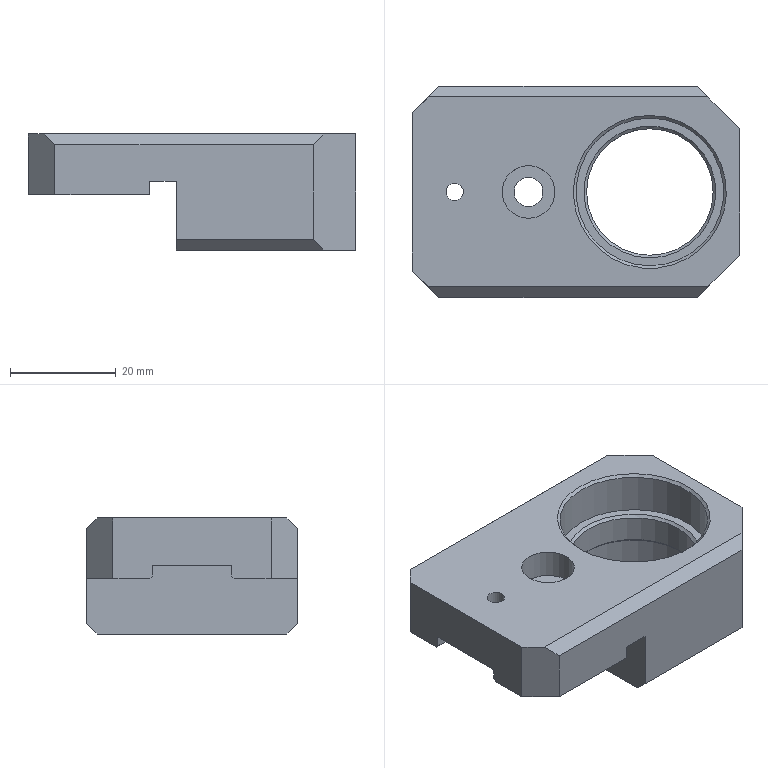Part | NX | 1 solid | 37 faces | box 62 x 40 x 22 mm | volume 26234 mm3 | plane 27 | cylinder 6 | cone 4 | commonest cylinder face diameters 28 x2 3.3 x1 5.5 x1 10 x1 24 x1
STEP:
#1=CARTESIAN_POINT('',(14.,-12.,-8.5));
#2=VERTEX_POINT('',#1);
#3=CARTESIAN_POINT('',(14.,0.,-8.5));
#4=DIRECTION('',(0.,0.,1.));
#5=DIRECTION('',(0.,-1.,0.));
#6=AXIS2_PLACEMENT_3D('',#3,#4,#5);
#7=CIRCLE('',#6,12.);
#8=EDGE_CURVE('',#2,#2,#7,.T.);
#9=ORIENTED_EDGE('',*,*,#8,.T.);
#10=EDGE_LOOP('',(#9));
#11=FACE_BOUND('',#10,.T.);
#12=CARTESIAN_POINT('',(14.,12.,-13.5));
#13=VERTEX_POINT('',#12);
#14=CARTESIAN_POINT('',(14.,0.,-13.5));
#15=DIRECTION('',(0.,0.,-1.));
#16=DIRECTION('',(0.,1.,0.));
#17=AXIS2_PLACEMENT_3D('',#14,#15,#16);
#18=CIRCLE('',#17,12.);
#19=EDGE_CURVE('',#13,#13,#18,.T.);
#20=ORIENTED_EDGE('',*,*,#19,.T.);
#21=EDGE_LOOP('',(#20));
#22=FACE_BOUND('',#21,.T.);
#23=CARTESIAN_POINT('',(14.,0.,-22.));
#24=DIRECTION('',(0.,0.,1.));
#25=DIRECTION('',(0.,-1.,0.));
#26=AXIS2_PLACEMENT_3D('',#23,#24,#25);
#27=CYLINDRICAL_SURFACE('',#26,12.);
#28=ADVANCED_FACE('',(#11,#22),#27,.F.);
#29=CARTESIAN_POINT('',(14.,-14.5,-22.));
#30=VERTEX_POINT('',#29);
#31=CARTESIAN_POINT('',(14.,0.,-22.));
#32=DIRECTION('',(0.,0.,1.));
#33=DIRECTION('',(0.,-1.,0.));
#34=AXIS2_PLACEMENT_3D('',#31,#32,#33);
#35=CIRCLE('',#34,14.5);
#36=EDGE_CURVE('',#30,#30,#35,.T.);
#37=ORIENTED_EDGE('',*,*,#36,.T.);
#38=EDGE_LOOP('',(#37));
#39=FACE_BOUND('',#38,.T.);
#40=CARTESIAN_POINT('',(31.,-12.,-22.));
#41=VERTEX_POINT('',#40);
#42=CARTESIAN_POINT('',(31.,12.,-22.));
#43=VERTEX_POINT('',#42);
#44=CARTESIAN_POINT('',(31.,-20.,-22.));
#45=DIRECTION('',(0.,1.,0.));
#46=VECTOR('',#45,1000.);
#47=LINE('',#44,#46);
#48=EDGE_CURVE('',#41,#43,#47,.T.);
#49=ORIENTED_EDGE('',*,*,#48,.F.);
#50=CARTESIAN_POINT('',(25.,-18.,-22.));
#51=VERTEX_POINT('',#50);
#52=CARTESIAN_POINT('',(31.,-12.,-22.));
#53=DIRECTION('',(0.7071,0.7071,0.));
#54=VECTOR('',#53,1000.);
#55=LINE('',#52,#54);
#56=EDGE_CURVE('',#41,#51,#55,.F.);
#57=ORIENTED_EDGE('',*,*,#56,.T.);
#58=CARTESIAN_POINT('',(-3.,-18.,-22.));
#59=VERTEX_POINT('',#58);
#60=CARTESIAN_POINT('',(31.,-18.,-22.));
#61=DIRECTION('',(-1.,0.,0.));
#62=VECTOR('',#61,1000.);
#63=LINE('',#60,#62);
#64=EDGE_CURVE('',#51,#59,#63,.T.);
#65=ORIENTED_EDGE('',*,*,#64,.T.);
#66=CARTESIAN_POINT('',(-3.,18.,-22.));
#67=VERTEX_POINT('',#66);
#68=CARTESIAN_POINT('',(-3.,-20.,-22.));
#69=DIRECTION('',(0.,-1.,0.));
#70=VECTOR('',#69,1000.);
#71=LINE('',#68,#70);
#72=EDGE_CURVE('',#67,#59,#71,.T.);
#73=ORIENTED_EDGE('',*,*,#72,.F.);
#74=CARTESIAN_POINT('',(25.,18.,-22.));
#75=VERTEX_POINT('',#74);
#76=CARTESIAN_POINT('',(31.,18.,-22.));
#77=DIRECTION('',(1.,0.,0.));
#78=VECTOR('',#77,1000.);
#79=LINE('',#76,#78);
#80=EDGE_CURVE('',#67,#75,#79,.T.);
#81=ORIENTED_EDGE('',*,*,#80,.T.);
#82=CARTESIAN_POINT('',(31.,12.,-22.));
#83=DIRECTION('',(-0.7071,0.7071,0.));
#84=VECTOR('',#83,1000.);
#85=LINE('',#82,#84);
#86=EDGE_CURVE('',#75,#43,#85,.F.);
#87=ORIENTED_EDGE('',*,*,#86,.T.);
#88=EDGE_LOOP('',(#49,#57,#65,#73,#81,#87));
#89=FACE_BOUND('',#88,.T.);
#90=CARTESIAN_POINT('',(31.,-20.,-22.));
#91=DIRECTION('',(0.,0.,1.));
#92=DIRECTION('',(0.,-1.,0.));
#93=AXIS2_PLACEMENT_3D('',#90,#91,#92);
#94=PLANE('',#93);
#95=ADVANCED_FACE('',(#39,#89),#94,.F.);
#96=CARTESIAN_POINT('',(23.,20.,-20.));
#97=VERTEX_POINT('',#96);
#98=CARTESIAN_POINT('',(-3.,20.,-20.));
#99=VERTEX_POINT('',#98);
#100=CARTESIAN_POINT('',(31.,20.,-20.));
#101=DIRECTION('',(-1.,0.,0.));
#102=VECTOR('',#101,1000.);
#103=LINE('',#100,#102);
#104=EDGE_CURVE('',#97,#99,#103,.T.);
#105=ORIENTED_EDGE('',*,*,#104,.F.);
#106=CARTESIAN_POINT('',(25.667,17.333,-22.667));
#107=DIRECTION('',(0.5774,-0.5774,-0.5774));
#108=VECTOR('',#107,1000.);
#109=LINE('',#106,#108);
#110=EDGE_CURVE('',#97,#75,#109,.T.);
#111=ORIENTED_EDGE('',*,*,#110,.T.);
#112=ORIENTED_EDGE('',*,*,#80,.F.);
#113=CARTESIAN_POINT('',(-3.,20.,-20.));
#114=DIRECTION('',(0.,-0.7071,-0.7071));
#115=VECTOR('',#114,1000.);
#116=LINE('',#113,#115);
#117=EDGE_CURVE('',#67,#99,#116,.F.);
#118=ORIENTED_EDGE('',*,*,#117,.T.);
#119=EDGE_LOOP('',(#105,#111,#112,#118));
#120=FACE_BOUND('',#119,.T.);
#121=CARTESIAN_POINT('',(31.,20.,-20.));
#122=DIRECTION('',(0.,-0.7071,0.7071));
#123=DIRECTION('',(-1.,0.,0.));
#124=AXIS2_PLACEMENT_3D('',#121,#122,#123);
#125=PLANE('',#124);
#126=ADVANCED_FACE('',(#120),#125,.F.);
#127=ORIENTED_EDGE('',*,*,#64,.F.);
#128=CARTESIAN_POINT('',(23.,-20.,-20.));
#129=VERTEX_POINT('',#128);
#130=CARTESIAN_POINT('',(27.,-16.,-24.));
#131=DIRECTION('',(-0.5774,-0.5774,0.5774));
#132=VECTOR('',#131,1000.);
#133=LINE('',#130,#132);
#134=EDGE_CURVE('',#51,#129,#133,.T.);
#135=ORIENTED_EDGE('',*,*,#134,.T.);
#136=CARTESIAN_POINT('',(-3.,-20.,-20.));
#137=VERTEX_POINT('',#136);
#138=CARTESIAN_POINT('',(31.,-20.,-20.));
#139=DIRECTION('',(1.,0.,0.));
#140=VECTOR('',#139,1000.);
#141=LINE('',#138,#140);
#142=EDGE_CURVE('',#137,#129,#141,.T.);
#143=ORIENTED_EDGE('',*,*,#142,.F.);
#144=CARTESIAN_POINT('',(-3.,-18.,-22.));
#145=DIRECTION('',(0.,-0.7071,0.7071));
#146=VECTOR('',#145,1000.);
#147=LINE('',#144,#146);
#148=EDGE_CURVE('',#137,#59,#147,.F.);
#149=ORIENTED_EDGE('',*,*,#148,.T.);
#150=EDGE_LOOP('',(#127,#135,#143,#149));
#151=FACE_BOUND('',#150,.T.);
#152=CARTESIAN_POINT('',(31.,-18.,-22.));
#153=DIRECTION('',(0.,0.7071,0.7071));
#154=DIRECTION('',(-1.,0.,0.));
#155=AXIS2_PLACEMENT_3D('',#152,#153,#154);
#156=PLANE('',#155);
#157=ADVANCED_FACE('',(#151),#156,.F.);
#158=CARTESIAN_POINT('',(-31.,-7.5,-9.));
#159=VERTEX_POINT('',#158);
#160=CARTESIAN_POINT('',(-31.,-7.5,-11.));
#161=VERTEX_POINT('',#160);
#162=CARTESIAN_POINT('',(-31.,-7.5,-35.));
#163=DIRECTION('',(0.,0.,-1.));
#164=VECTOR('',#163,1000.);
#165=LINE('',#162,#164);
#166=EDGE_CURVE('',#159,#161,#165,.T.);
#167=ORIENTED_EDGE('',*,*,#166,.T.);
#168=CARTESIAN_POINT('',(-31.,-8.,-11.5));
#169=VERTEX_POINT('',#168);
#170=CARTESIAN_POINT('',(-31.,-3.75,-7.25));
#171=DIRECTION('',(0.,-0.7071,-0.7071));
#172=VECTOR('',#171,1000.);
#173=LINE('',#170,#172);
#174=EDGE_CURVE('',#161,#169,#173,.T.);
#175=ORIENTED_EDGE('',*,*,#174,.T.);
#176=CARTESIAN_POINT('',(-31.,-15.,-11.5));
#177=VERTEX_POINT('',#176);
#178=CARTESIAN_POINT('',(-31.,-20.,-11.5));
#179=DIRECTION('',(0.,1.,0.));
#180=VECTOR('',#179,1000.);
#181=LINE('',#178,#180);
#182=EDGE_CURVE('',#177,#169,#181,.T.);
#183=ORIENTED_EDGE('',*,*,#182,.F.);
#184=CARTESIAN_POINT('',(-31.,-15.,0.));
#185=VERTEX_POINT('',#184);
#186=CARTESIAN_POINT('',(-31.,-15.,-2.));
#187=DIRECTION('',(0.,0.,1.));
#188=VECTOR('',#187,1000.);
#189=LINE('',#186,#188);
#190=EDGE_CURVE('',#177,#185,#189,.T.);
#191=ORIENTED_EDGE('',*,*,#190,.T.);
#192=CARTESIAN_POINT('',(-31.,15.,0.));
#193=VERTEX_POINT('',#192);
#194=CARTESIAN_POINT('',(-31.,-20.,0.));
#195=DIRECTION('',(0.,-1.,0.));
#196=VECTOR('',#195,1000.);
#197=LINE('',#194,#196);
#198=EDGE_CURVE('',#193,#185,#197,.T.);
#199=ORIENTED_EDGE('',*,*,#198,.F.);
#200=CARTESIAN_POINT('',(-31.,15.,-11.5));
#201=VERTEX_POINT('',#200);
#202=CARTESIAN_POINT('',(-31.,15.,-13.5));
#203=DIRECTION('',(0.,0.,-1.));
#204=VECTOR('',#203,1000.);
#205=LINE('',#202,#204);
#206=EDGE_CURVE('',#193,#201,#205,.T.);
#207=ORIENTED_EDGE('',*,*,#206,.T.);
#208=CARTESIAN_POINT('',(-31.,8.,-11.5));
#209=VERTEX_POINT('',#208);
#210=CARTESIAN_POINT('',(-31.,-20.,-11.5));
#211=DIRECTION('',(0.,1.,0.));
#212=VECTOR('',#211,1000.);
#213=LINE('',#210,#212);
#214=EDGE_CURVE('',#209,#201,#213,.T.);
#215=ORIENTED_EDGE('',*,*,#214,.F.);
#216=CARTESIAN_POINT('',(-31.,7.5,-11.));
#217=VERTEX_POINT('',#216);
#218=CARTESIAN_POINT('',(-31.,3.75,-7.25));
#219=DIRECTION('',(0.,-0.7071,0.7071));
#220=VECTOR('',#219,1000.);
#221=LINE('',#218,#220);
#222=EDGE_CURVE('',#209,#217,#221,.T.);
#223=ORIENTED_EDGE('',*,*,#222,.T.);
#224=CARTESIAN_POINT('',(-31.,7.5,-9.));
#225=VERTEX_POINT('',#224);
#226=CARTESIAN_POINT('',(-31.,7.5,-11.));
#227=DIRECTION('',(0.,0.,1.));
#228=VECTOR('',#227,1000.);
#229=LINE('',#226,#228);
#230=EDGE_CURVE('',#217,#225,#229,.T.);
#231=ORIENTED_EDGE('',*,*,#230,.T.);
#232=CARTESIAN_POINT('',(-31.,-7.5,-9.));
#233=DIRECTION('',(0.,-1.,0.));
#234=VECTOR('',#233,1000.);
#235=LINE('',#232,#234);
#236=EDGE_CURVE('',#225,#159,#235,.T.);
#237=ORIENTED_EDGE('',*,*,#236,.T.);
#238=EDGE_LOOP('',(#167,#175,#183,#191,#199,#207,#215,#223,#231,#237));
#239=FACE_BOUND('',#238,.T.);
#240=CARTESIAN_POINT('',(-31.,0.,-11.));
#241=DIRECTION('',(-1.,0.,0.));
#242=DIRECTION('',(0.,0.,1.));
#243=AXIS2_PLACEMENT_3D('',#240,#241,#242);
#244=PLANE('',#243);
#245=ADVANCED_FACE('',(#239),#244,.T.);
#246=CARTESIAN_POINT('',(-8.,20.,-9.));
#247=VERTEX_POINT('',#246);
#248=CARTESIAN_POINT('',(-8.,20.,-11.5));
#249=VERTEX_POINT('',#248);
#250=CARTESIAN_POINT('',(-8.,20.,31.311));
#251=DIRECTION('',(0.,0.,-1.));
#252=VECTOR('',#251,1000.);
#253=LINE('',#250,#252);
#254=EDGE_CURVE('',#247,#249,#253,.T.);
#255=ORIENTED_EDGE('',*,*,#254,.T.);
#256=CARTESIAN_POINT('',(-26.,20.,-11.5));
#257=VERTEX_POINT('',#256);
#258=CARTESIAN_POINT('',(37.112,20.,-11.5));
#259=DIRECTION('',(-1.,0.,0.));
#260=VECTOR('',#259,1000.);
#261=LINE('',#258,#260);
#262=EDGE_CURVE('',#249,#257,#261,.T.);
#263=ORIENTED_EDGE('',*,*,#262,.T.);
#264=CARTESIAN_POINT('',(-26.,20.,-2.));
#265=VERTEX_POINT('',#264);
#266=CARTESIAN_POINT('',(-26.,20.,-2.));
#267=DIRECTION('',(0.,0.,1.));
#268=VECTOR('',#267,1000.);
#269=LINE('',#266,#268);
#270=EDGE_CURVE('',#257,#265,#269,.T.);
#271=ORIENTED_EDGE('',*,*,#270,.T.);
#272=CARTESIAN_POINT('',(23.,20.,-2.));
#273=VERTEX_POINT('',#272);
#274=CARTESIAN_POINT('',(31.,20.,-2.));
#275=DIRECTION('',(1.,0.,0.));
#276=VECTOR('',#275,1000.);
#277=LINE('',#274,#276);
#278=EDGE_CURVE('',#265,#273,#277,.T.);
#279=ORIENTED_EDGE('',*,*,#278,.T.);
#280=CARTESIAN_POINT('',(23.,20.,-22.));
#281=DIRECTION('',(0.,0.,-1.));
#282=VECTOR('',#281,1000.);
#283=LINE('',#280,#282);
#284=EDGE_CURVE('',#273,#97,#283,.T.);
#285=ORIENTED_EDGE('',*,*,#284,.T.);
#286=ORIENTED_EDGE('',*,*,#104,.T.);
#287=CARTESIAN_POINT('',(-3.,20.,-9.));
#288=VERTEX_POINT('',#287);
#289=CARTESIAN_POINT('',(-3.,20.,-14.));
#290=DIRECTION('',(0.,0.,1.));
#291=VECTOR('',#290,1000.);
#292=LINE('',#289,#291);
#293=EDGE_CURVE('',#99,#288,#292,.T.);
#294=ORIENTED_EDGE('',*,*,#293,.T.);
#295=CARTESIAN_POINT('',(-3.,20.,-9.));
#296=DIRECTION('',(-1.,0.,0.));
#297=VECTOR('',#296,1000.);
#298=LINE('',#295,#297);
#299=EDGE_CURVE('',#288,#247,#298,.T.);
#300=ORIENTED_EDGE('',*,*,#299,.T.);
#301=EDGE_LOOP('',(#255,#263,#271,#279,#285,#286,#294,#300));
#302=FACE_BOUND('',#301,.T.);
#303=CARTESIAN_POINT('',(31.,20.,-22.));
#304=DIRECTION('',(0.,-1.,0.));
#305=DIRECTION('',(0.,0.,-1.));
#306=AXIS2_PLACEMENT_3D('',#303,#304,#305);
#307=PLANE('',#306);
#308=ADVANCED_FACE('',(#302),#307,.F.);
#309=CARTESIAN_POINT('',(-9.,-5.,0.));
#310=VERTEX_POINT('',#309);
#311=CARTESIAN_POINT('',(-9.,0.,0.));
#312=DIRECTION('',(0.,0.,1.));
#313=DIRECTION('',(0.,-1.,0.));
#314=AXIS2_PLACEMENT_3D('',#311,#312,#313);
#315=CIRCLE('',#314,5.);
#316=EDGE_CURVE('',#310,#310,#315,.T.);
#317=ORIENTED_EDGE('',*,*,#316,.F.);
#318=EDGE_LOOP('',(#317));
#319=FACE_BOUND('',#318,.T.);
#320=CARTESIAN_POINT('',(14.,14.5,0.));
#321=VERTEX_POINT('',#320);
#322=CARTESIAN_POINT('',(14.,0.,0.));
#323=DIRECTION('',(0.,0.,-1.));
#324=DIRECTION('',(0.,1.,0.));
#325=AXIS2_PLACEMENT_3D('',#322,#323,#324);
#326=CIRCLE('',#325,14.5);
#327=EDGE_CURVE('',#321,#321,#326,.T.);
#328=ORIENTED_EDGE('',*,*,#327,.T.);
#329=EDGE_LOOP('',(#328));
#330=FACE_BOUND('',#329,.T.);
#331=CARTESIAN_POINT('',(-23.,1.65,0.));
#332=VERTEX_POINT('',#331);
#333=CARTESIAN_POINT('',(-23.,0.,0.));
#334=DIRECTION('',(0.,0.,-1.));
#335=DIRECTION('',(0.,1.,0.));
#336=AXIS2_PLACEMENT_3D('',#333,#334,#335);
#337=CIRCLE('',#336,1.65);
#338=EDGE_CURVE('',#332,#332,#337,.T.);
#339=ORIENTED_EDGE('',*,*,#338,.T.);
#340=EDGE_LOOP('',(#339));
#341=FACE_BOUND('',#340,.T.);
#342=ORIENTED_EDGE('',*,*,#198,.T.);
#343=CARTESIAN_POINT('',(-28.,-18.,0.));
#344=VERTEX_POINT('',#343);
#345=CARTESIAN_POINT('',(-26.,-20.,0.));
#346=DIRECTION('',(0.7071,-0.7071,0.));
#347=VECTOR('',#346,1000.);
#348=LINE('',#345,#347);
#349=EDGE_CURVE('',#185,#344,#348,.T.);
#350=ORIENTED_EDGE('',*,*,#349,.T.);
#351=CARTESIAN_POINT('',(25.,-18.,0.));
#352=VERTEX_POINT('',#351);
#353=CARTESIAN_POINT('',(31.,-18.,0.));
#354=DIRECTION('',(1.,0.,0.));
#355=VECTOR('',#354,1000.);
#356=LINE('',#353,#355);
#357=EDGE_CURVE('',#344,#352,#356,.T.);
#358=ORIENTED_EDGE('',*,*,#357,.T.);
#359=CARTESIAN_POINT('',(31.,-12.,0.));
#360=VERTEX_POINT('',#359);
#361=CARTESIAN_POINT('',(31.,-12.,0.));
#362=DIRECTION('',(-0.7071,-0.7071,0.));
#363=VECTOR('',#362,1000.);
#364=LINE('',#361,#363);
#365=EDGE_CURVE('',#352,#360,#364,.F.);
#366=ORIENTED_EDGE('',*,*,#365,.T.);
#367=CARTESIAN_POINT('',(31.,12.,0.));
#368=VERTEX_POINT('',#367);
#369=CARTESIAN_POINT('',(31.,-20.,0.));
#370=DIRECTION('',(0.,-1.,0.));
#371=VECTOR('',#370,1000.);
#372=LINE('',#369,#371);
#373=EDGE_CURVE('',#368,#360,#372,.T.);
#374=ORIENTED_EDGE('',*,*,#373,.F.);
#375=CARTESIAN_POINT('',(25.,18.,0.));
#376=VERTEX_POINT('',#375);
#377=CARTESIAN_POINT('',(31.,12.,0.));
#378=DIRECTION('',(0.7071,-0.7071,0.));
#379=VECTOR('',#378,1000.);
#380=LINE('',#377,#379);
#381=EDGE_CURVE('',#368,#376,#380,.F.);
#382=ORIENTED_EDGE('',*,*,#381,.T.);
#383=CARTESIAN_POINT('',(-28.,18.,0.));
#384=VERTEX_POINT('',#383);
#385=CARTESIAN_POINT('',(31.,18.,0.));
#386=DIRECTION('',(-1.,0.,0.));
#387=VECTOR('',#386,1000.);
#388=LINE('',#385,#387);
#389=EDGE_CURVE('',#376,#384,#388,.T.);
#390=ORIENTED_EDGE('',*,*,#389,.T.);
#391=CARTESIAN_POINT('',(-26.,20.,0.));
#392=DIRECTION('',(-0.7071,-0.7071,0.));
#393=VECTOR('',#392,1000.);
#394=LINE('',#391,#393);
#395=EDGE_CURVE('',#384,#193,#394,.T.);
#396=ORIENTED_EDGE('',*,*,#395,.T.);
#397=EDGE_LOOP('',(#342,#350,#358,#366,#374,#382,#390,#396));
#398=FACE_BOUND('',#397,.T.);
#399=CARTESIAN_POINT('',(31.,-20.,0.));
#400=DIRECTION('',(0.,0.,-1.));
#401=DIRECTION('',(0.,1.,0.));
#402=AXIS2_PLACEMENT_3D('',#399,#400,#401);
#403=PLANE('',#402);
#404=ADVANCED_FACE('',(#319,#330,#341,#398),#403,.F.);
#405=CARTESIAN_POINT('',(-26.,-20.,-2.));
#406=VERTEX_POINT('',#405);
#407=CARTESIAN_POINT('',(-26.,-20.,-11.5));
#408=VERTEX_POINT('',#407);
#409=CARTESIAN_POINT('',(-26.,-20.,-13.5));
#410=DIRECTION('',(0.,0.,-1.));
#411=VECTOR('',#410,1000.);
#412=LINE('',#409,#411);
#413=EDGE_CURVE('',#406,#408,#412,.T.);
#414=ORIENTED_EDGE('',*,*,#413,.T.);
#415=CARTESIAN_POINT('',(-8.,-20.,-11.5));
#416=VERTEX_POINT('',#415);
#417=CARTESIAN_POINT('',(37.112,-20.,-11.5));
#418=DIRECTION('',(-1.,0.,0.));
#419=VECTOR('',#418,1000.);
#420=LINE('',#417,#419);
#421=EDGE_CURVE('',#416,#408,#420,.T.);
#422=ORIENTED_EDGE('',*,*,#421,.F.);
#423=CARTESIAN_POINT('',(-8.,-20.,-9.));
#424=VERTEX_POINT('',#423);
#425=CARTESIAN_POINT('',(-8.,-20.,31.311));
#426=DIRECTION('',(0.,0.,-1.));
#427=VECTOR('',#426,1000.);
#428=LINE('',#425,#427);
#429=EDGE_CURVE('',#424,#416,#428,.T.);
#430=ORIENTED_EDGE('',*,*,#429,.F.);
#431=CARTESIAN_POINT('',(-3.,-20.,-9.));
#432=VERTEX_POINT('',#431);
#433=CARTESIAN_POINT('',(-3.,-20.,-9.));
#434=DIRECTION('',(1.,0.,0.));
#435=VECTOR('',#434,1000.);
#436=LINE('',#433,#435);
#437=EDGE_CURVE('',#424,#432,#436,.T.);
#438=ORIENTED_EDGE('',*,*,#437,.T.);
#439=CARTESIAN_POINT('',(-3.,-20.,-14.));
#440=DIRECTION('',(0.,0.,-1.));
#441=VECTOR('',#440,1000.);
#442=LINE('',#439,#441);
#443=EDGE_CURVE('',#432,#137,#442,.T.);
#444=ORIENTED_EDGE('',*,*,#443,.T.);
#445=ORIENTED_EDGE('',*,*,#142,.T.);
#446=CARTESIAN_POINT('',(23.,-20.,-2.));
#447=VERTEX_POINT('',#446);
#448=CARTESIAN_POINT('',(23.,-20.,-22.));
#449=DIRECTION('',(0.,0.,1.));
#450=VECTOR('',#449,1000.);
#451=LINE('',#448,#450);
#452=EDGE_CURVE('',#129,#447,#451,.T.);
#453=ORIENTED_EDGE('',*,*,#452,.T.);
#454=CARTESIAN_POINT('',(31.,-20.,-2.));
#455=DIRECTION('',(-1.,0.,0.));
#456=VECTOR('',#455,1000.);
#457=LINE('',#454,#456);
#458=EDGE_CURVE('',#447,#406,#457,.T.);
#459=ORIENTED_EDGE('',*,*,#458,.T.);
#460=EDGE_LOOP('',(#414,#422,#430,#438,#444,#445,#453,#459));
#461=FACE_BOUND('',#460,.T.);
#462=CARTESIAN_POINT('',(31.,-20.,-22.));
#463=DIRECTION('',(0.,1.,0.));
#464=DIRECTION('',(0.,0.,1.));
#465=AXIS2_PLACEMENT_3D('',#462,#463,#464);
#466=PLANE('',#465);
#467=ADVANCED_FACE('',(#461),#466,.F.);
#468=ORIENTED_EDGE('',*,*,#373,.T.);
#469=CARTESIAN_POINT('',(31.,-12.,-11.));
#470=DIRECTION('',(0.,0.,-1.));
#471=VECTOR('',#470,1000.);
#472=LINE('',#469,#471);
#473=EDGE_CURVE('',#360,#41,#472,.T.);
#474=ORIENTED_EDGE('',*,*,#473,.T.);
#475=ORIENTED_EDGE('',*,*,#48,.T.);
#476=CARTESIAN_POINT('',(31.,12.,-11.));
#477=DIRECTION('',(0.,0.,1.));
#478=VECTOR('',#477,1000.);
#479=LINE('',#476,#478);
#480=EDGE_CURVE('',#43,#368,#479,.T.);
#481=ORIENTED_EDGE('',*,*,#480,.T.);
#482=EDGE_LOOP('',(#468,#474,#475,#481));
#483=FACE_BOUND('',#482,.T.);
#484=CARTESIAN_POINT('',(31.,0.,-11.));
#485=DIRECTION('',(-1.,0.,0.));
#486=DIRECTION('',(0.,0.,1.));
#487=AXIS2_PLACEMENT_3D('',#484,#485,#486);
#488=PLANE('',#487);
#489=ADVANCED_FACE('',(#483),#488,.F.);
#490=ORIENTED_EDGE('',*,*,#357,.F.);
#491=CARTESIAN_POINT('',(-7.,-39.,-21.));
#492=DIRECTION('',(-0.5774,0.5774,0.5774));
#493=VECTOR('',#492,1000.);
#494=LINE('',#491,#493);
#495=EDGE_CURVE('',#344,#406,#494,.F.);
#496=ORIENTED_EDGE('',*,*,#495,.T.);
#497=ORIENTED_EDGE('',*,*,#458,.F.);
#498=CARTESIAN_POINT('',(25.667,-17.333,0.6667));
#499=DIRECTION('',(0.5774,0.5774,0.5774));
#500=VECTOR('',#499,1000.);
#501=LINE('',#498,#500);
#502=EDGE_CURVE('',#447,#352,#501,.T.);
#503=ORIENTED_EDGE('',*,*,#502,.T.);
#504=EDGE_LOOP('',(#490,#496,#497,#503));
#505=FACE_BOUND('',#504,.T.);
#506=CARTESIAN_POINT('',(31.,-20.,-2.));
#507=DIRECTION('',(0.,0.7071,-0.7071));
#508=DIRECTION('',(-1.,0.,0.));
#509=AXIS2_PLACEMENT_3D('',#506,#507,#508);
#510=PLANE('',#509);
#511=ADVANCED_FACE('',(#505),#510,.F.);
#512=ORIENTED_EDGE('',*,*,#278,.F.);
#513=CARTESIAN_POINT('',(-8.333,37.667,-19.667));
#514=DIRECTION('',(0.5774,0.5774,-0.5774));
#515=VECTOR('',#514,1000.);
#516=LINE('',#513,#515);
#517=EDGE_CURVE('',#265,#384,#516,.F.);
#518=ORIENTED_EDGE('',*,*,#517,.T.);
#519=ORIENTED_EDGE('',*,*,#389,.F.);
#520=CARTESIAN_POINT('',(27.,16.,2.));
#521=DIRECTION('',(-0.5774,0.5774,-0.5774));
#522=VECTOR('',#521,1000.);
#523=LINE('',#520,#522);
#524=EDGE_CURVE('',#376,#273,#523,.T.);
#525=ORIENTED_EDGE('',*,*,#524,.T.);
#526=EDGE_LOOP('',(#512,#518,#519,#525));
#527=FACE_BOUND('',#526,.T.);
#528=CARTESIAN_POINT('',(31.,18.,0.));
#529=DIRECTION('',(0.,-0.7071,-0.7071));
#530=DIRECTION('',(-1.,0.,0.));
#531=AXIS2_PLACEMENT_3D('',#528,#529,#530);
#532=PLANE('',#531);
#533=ADVANCED_FACE('',(#527),#532,.F.);
#534=CARTESIAN_POINT('',(-3.,-7.5,-9.));
#535=DIRECTION('',(0.,-1.,0.));
#536=VECTOR('',#535,1000.);
#537=LINE('',#534,#536);
#538=EDGE_CURVE('',#288,#432,#537,.T.);
#539=ORIENTED_EDGE('',*,*,#538,.F.);
#540=ORIENTED_EDGE('',*,*,#293,.F.);
#541=ORIENTED_EDGE('',*,*,#117,.F.);
#542=ORIENTED_EDGE('',*,*,#72,.T.);
#543=ORIENTED_EDGE('',*,*,#148,.F.);
#544=ORIENTED_EDGE('',*,*,#443,.F.);
#545=EDGE_LOOP('',(#539,#540,#541,#542,#543,#544));
#546=FACE_BOUND('',#545,.T.);
#547=CARTESIAN_POINT('',(-3.,0.,-11.));
#548=DIRECTION('',(-1.,0.,0.));
#549=DIRECTION('',(0.,0.,1.));
#550=AXIS2_PLACEMENT_3D('',#547,#548,#549);
#551=PLANE('',#550);
#552=ADVANCED_FACE('',(#546),#551,.T.);
#553=ORIENTED_EDGE('',*,*,#230,.F.);
#554=CARTESIAN_POINT('',(-8.,7.5,-11.));
#555=VERTEX_POINT('',#554);
#556=CARTESIAN_POINT('',(-8.,7.5,-11.));
#557=DIRECTION('',(1.,0.,0.));
#558=VECTOR('',#557,1000.);
#559=LINE('',#556,#558);
#560=EDGE_CURVE('',#217,#555,#559,.T.);
#561=ORIENTED_EDGE('',*,*,#560,.T.);
#562=CARTESIAN_POINT('',(-8.,7.5,-9.));
#563=VERTEX_POINT('',#562);
#564=CARTESIAN_POINT('',(-8.,7.5,-35.));
#565=DIRECTION('',(0.,0.,-1.));
#566=VECTOR('',#565,1000.);
#567=LINE('',#564,#566);
#568=EDGE_CURVE('',#563,#555,#567,.T.);
#569=ORIENTED_EDGE('',*,*,#568,.F.);
#570=CARTESIAN_POINT('',(-3.,7.5,-9.));
#571=DIRECTION('',(-1.,0.,0.));
#572=VECTOR('',#571,1000.);
#573=LINE('',#570,#572);
#574=EDGE_CURVE('',#563,#225,#573,.T.);
#575=ORIENTED_EDGE('',*,*,#574,.T.);
#576=EDGE_LOOP('',(#553,#561,#569,#575));
#577=FACE_BOUND('',#576,.T.);
#578=CARTESIAN_POINT('',(-3.,7.5,-35.));
#579=DIRECTION('',(0.,-1.,0.));
#580=DIRECTION('',(0.,0.,-1.));
#581=AXIS2_PLACEMENT_3D('',#578,#579,#580);
#582=PLANE('',#581);
#583=ADVANCED_FACE('',(#577),#582,.T.);
#584=CARTESIAN_POINT('',(-8.,-7.5,-11.));
#585=VERTEX_POINT('',#584);
#586=CARTESIAN_POINT('',(-8.,-7.5,-9.));
#587=VERTEX_POINT('',#586);
#588=CARTESIAN_POINT('',(-8.,-7.5,-35.));
#589=DIRECTION('',(0.,0.,1.));
#590=VECTOR('',#589,1000.);
#591=LINE('',#588,#590);
#592=EDGE_CURVE('',#585,#587,#591,.T.);
#593=ORIENTED_EDGE('',*,*,#592,.F.);
#594=CARTESIAN_POINT('',(-31.,-7.5,-11.));
#595=DIRECTION('',(-1.,0.,0.));
#596=VECTOR('',#595,1000.);
#597=LINE('',#594,#596);
#598=EDGE_CURVE('',#585,#161,#597,.T.);
#599=ORIENTED_EDGE('',*,*,#598,.T.);
#600=ORIENTED_EDGE('',*,*,#166,.F.);
#601=CARTESIAN_POINT('',(-3.,-7.5,-9.));
#602=DIRECTION('',(-1.,0.,0.));
#603=VECTOR('',#602,1000.);
#604=LINE('',#601,#603);
#605=EDGE_CURVE('',#587,#159,#604,.T.);
#606=ORIENTED_EDGE('',*,*,#605,.F.);
#607=EDGE_LOOP('',(#593,#599,#600,#606));
#608=FACE_BOUND('',#607,.T.);
#609=CARTESIAN_POINT('',(-3.,-7.5,-35.));
#610=DIRECTION('',(0.,1.,0.));
#611=DIRECTION('',(0.,0.,1.));
#612=AXIS2_PLACEMENT_3D('',#609,#610,#611);
#613=PLANE('',#612);
#614=ADVANCED_FACE('',(#608),#613,.T.);
#615=CARTESIAN_POINT('',(-9.,2.75,-9.));
#616=VERTEX_POINT('',#615);
#617=CARTESIAN_POINT('',(-9.,0.,-9.));
#618=DIRECTION('',(0.,0.,-1.));
#619=DIRECTION('',(0.,1.,0.));
#620=AXIS2_PLACEMENT_3D('',#617,#618,#619);
#621=CIRCLE('',#620,2.75);
#622=EDGE_CURVE('',#616,#616,#621,.T.);
#623=ORIENTED_EDGE('',*,*,#622,.F.);
#624=EDGE_LOOP('',(#623));
#625=FACE_BOUND('',#624,.T.);
#626=ORIENTED_EDGE('',*,*,#574,.F.);
#627=CARTESIAN_POINT('',(-8.,-20.,-9.));
#628=DIRECTION('',(0.,-1.,0.));
#629=VECTOR('',#628,1000.);
#630=LINE('',#627,#629);
#631=EDGE_CURVE('',#247,#563,#630,.T.);
#632=ORIENTED_EDGE('',*,*,#631,.F.);
#633=ORIENTED_EDGE('',*,*,#299,.F.);
#634=ORIENTED_EDGE('',*,*,#538,.T.);
#635=ORIENTED_EDGE('',*,*,#437,.F.);
#636=CARTESIAN_POINT('',(-8.,-20.,-9.));
#637=DIRECTION('',(0.,-1.,0.));
#638=VECTOR('',#637,1000.);
#639=LINE('',#636,#638);
#640=EDGE_CURVE('',#587,#424,#639,.T.);
#641=ORIENTED_EDGE('',*,*,#640,.F.);
#642=ORIENTED_EDGE('',*,*,#605,.T.);
#643=ORIENTED_EDGE('',*,*,#236,.F.);
#644=EDGE_LOOP('',(#626,#632,#633,#634,#635,#641,#642,#643));
#645=FACE_BOUND('',#644,.T.);
#646=CARTESIAN_POINT('',(-23.,1.65,-9.));
#647=VERTEX_POINT('',#646);
#648=CARTESIAN_POINT('',(-23.,0.,-9.));
#649=DIRECTION('',(0.,0.,-1.));
#650=DIRECTION('',(0.,1.,0.));
#651=AXIS2_PLACEMENT_3D('',#648,#649,#650);
#652=CIRCLE('',#651,1.65);
#653=EDGE_CURVE('',#647,#647,#652,.T.);
#654=ORIENTED_EDGE('',*,*,#653,.F.);
#655=EDGE_LOOP('',(#654));
#656=FACE_BOUND('',#655,.T.);
#657=CARTESIAN_POINT('',(-3.,-7.5,-9.));
#658=DIRECTION('',(0.,0.,-1.));
#659=DIRECTION('',(0.,1.,0.));
#660=AXIS2_PLACEMENT_3D('',#657,#658,#659);
#661=PLANE('',#660);
#662=ADVANCED_FACE('',(#625,#645,#656),#661,.T.);
#663=ORIENTED_EDGE('',*,*,#653,.T.);
#664=EDGE_LOOP('',(#663));
#665=FACE_BOUND('',#664,.T.);
#666=ORIENTED_EDGE('',*,*,#338,.F.);
#667=EDGE_LOOP('',(#666));
#668=FACE_BOUND('',#667,.T.);
#669=CARTESIAN_POINT('',(-23.,0.,-9.));
#670=DIRECTION('',(0.,0.,-1.));
#671=DIRECTION('',(0.,1.,0.));
#672=AXIS2_PLACEMENT_3D('',#669,#670,#671);
#673=CYLINDRICAL_SURFACE('',#672,1.65);
#674=ADVANCED_FACE('',(#665,#668),#673,.F.);
#675=ORIENTED_EDGE('',*,*,#568,.T.);
#676=CARTESIAN_POINT('',(-8.,8.,-11.5));
#677=VERTEX_POINT('',#676);
#678=CARTESIAN_POINT('',(-8.,8.,-11.5));
#679=DIRECTION('',(0.,0.7071,-0.7071));
#680=VECTOR('',#679,1000.);
#681=LINE('',#678,#680);
#682=EDGE_CURVE('',#555,#677,#681,.T.);
#683=ORIENTED_EDGE('',*,*,#682,.T.);
#684=CARTESIAN_POINT('',(-8.,-20.,-11.5));
#685=DIRECTION('',(0.,1.,0.));
#686=VECTOR('',#685,1000.);
#687=LINE('',#684,#686);
#688=EDGE_CURVE('',#677,#249,#687,.T.);
#689=ORIENTED_EDGE('',*,*,#688,.T.);
#690=ORIENTED_EDGE('',*,*,#254,.F.);
#691=ORIENTED_EDGE('',*,*,#631,.T.);
#692=EDGE_LOOP('',(#675,#683,#689,#690,#691));
#693=FACE_BOUND('',#692,.T.);
#694=CARTESIAN_POINT('',(-8.,-20.,31.311));
#695=DIRECTION('',(-1.,0.,0.));
#696=DIRECTION('',(0.,0.,1.));
#697=AXIS2_PLACEMENT_3D('',#694,#695,#696);
#698=PLANE('',#697);
#699=ADVANCED_FACE('',(#693),#698,.F.);
#700=CARTESIAN_POINT('',(-8.,-8.,-11.5));
#701=VERTEX_POINT('',#700);
#702=CARTESIAN_POINT('',(-8.,-20.,-11.5));
#703=DIRECTION('',(0.,1.,0.));
#704=VECTOR('',#703,1000.);
#705=LINE('',#702,#704);
#706=EDGE_CURVE('',#416,#701,#705,.T.);
#707=ORIENTED_EDGE('',*,*,#706,.T.);
#708=CARTESIAN_POINT('',(-8.,-8.,-11.5));
#709=DIRECTION('',(0.,0.7071,0.7071));
#710=VECTOR('',#709,1000.);
#711=LINE('',#708,#710);
#712=EDGE_CURVE('',#701,#585,#711,.T.);
#713=ORIENTED_EDGE('',*,*,#712,.T.);
#714=ORIENTED_EDGE('',*,*,#592,.T.);
#715=ORIENTED_EDGE('',*,*,#640,.T.);
#716=ORIENTED_EDGE('',*,*,#429,.T.);
#717=EDGE_LOOP('',(#707,#713,#714,#715,#716));
#718=FACE_BOUND('',#717,.T.);
#719=CARTESIAN_POINT('',(-8.,-20.,31.311));
#720=DIRECTION('',(-1.,0.,0.));
#721=DIRECTION('',(0.,0.,1.));
#722=AXIS2_PLACEMENT_3D('',#719,#720,#721);
#723=PLANE('',#722);
#724=ADVANCED_FACE('',(#718),#723,.F.);
#725=CARTESIAN_POINT('',(14.,12.5,-14.));
#726=VERTEX_POINT('',#725);
#727=CARTESIAN_POINT('',(14.,0.,-14.));
#728=DIRECTION('',(0.,0.,-1.));
#729=DIRECTION('',(0.,1.,0.));
#730=AXIS2_PLACEMENT_3D('',#727,#728,#729);
#731=CIRCLE('',#730,12.5);
#732=EDGE_CURVE('',#726,#726,#731,.F.);
#733=ORIENTED_EDGE('',*,*,#732,.T.);
#734=EDGE_LOOP('',(#733));
#735=FACE_BOUND('',#734,.T.);
#736=CARTESIAN_POINT('',(14.,14.,-14.));
#737=VERTEX_POINT('',#736);
#738=CARTESIAN_POINT('',(14.,0.,-14.));
#739=DIRECTION('',(0.,0.,-1.));
#740=DIRECTION('',(0.,1.,0.));
#741=AXIS2_PLACEMENT_3D('',#738,#739,#740);
#742=CIRCLE('',#741,14.);
#743=EDGE_CURVE('',#737,#737,#742,.T.);
#744=ORIENTED_EDGE('',*,*,#743,.T.);
#745=EDGE_LOOP('',(#744));
#746=FACE_BOUND('',#745,.T.);
#747=CARTESIAN_POINT('',(14.,0.,-14.));
#748=DIRECTION('',(0.,0.,-1.));
#749=DIRECTION('',(0.,1.,0.));
#750=AXIS2_PLACEMENT_3D('',#747,#748,#749);
#751=PLANE('',#750);
#752=ADVANCED_FACE('',(#735,#746),#751,.T.);
#753=CARTESIAN_POINT('',(14.,-14.,-21.5));
#754=VERTEX_POINT('',#753);
#755=CARTESIAN_POINT('',(14.,0.,-21.5));
#756=DIRECTION('',(0.,0.,1.));
#757=DIRECTION('',(0.,-1.,0.));
#758=AXIS2_PLACEMENT_3D('',#755,#756,#757);
#759=CIRCLE('',#758,14.);
#760=EDGE_CURVE('',#754,#754,#759,.F.);
#761=ORIENTED_EDGE('',*,*,#760,.T.);
#762=EDGE_LOOP('',(#761));
#763=FACE_BOUND('',#762,.T.);
#764=ORIENTED_EDGE('',*,*,#743,.F.);
#765=EDGE_LOOP('',(#764));
#766=FACE_BOUND('',#765,.T.);
#767=CARTESIAN_POINT('',(14.,0.,-14.));
#768=DIRECTION('',(0.,0.,-1.));
#769=DIRECTION('',(0.,1.,0.));
#770=AXIS2_PLACEMENT_3D('',#767,#768,#769);
#771=CYLINDRICAL_SURFACE('',#770,14.);
#772=ADVANCED_FACE('',(#763,#766),#771,.F.);
#773=CARTESIAN_POINT('',(14.,-12.5,-8.));
#774=VERTEX_POINT('',#773);
#775=CARTESIAN_POINT('',(14.,0.,-8.));
#776=DIRECTION('',(0.,0.,1.));
#777=DIRECTION('',(0.,-1.,0.));
#778=AXIS2_PLACEMENT_3D('',#775,#776,#777);
#779=CIRCLE('',#778,12.5);
#780=EDGE_CURVE('',#774,#774,#779,.F.);
#781=ORIENTED_EDGE('',*,*,#780,.T.);
#782=EDGE_LOOP('',(#781));
#783=FACE_BOUND('',#782,.T.);
#784=CARTESIAN_POINT('',(14.,-14.,-8.));
#785=VERTEX_POINT('',#784);
#786=CARTESIAN_POINT('',(14.,0.,-8.));
#787=DIRECTION('',(0.,0.,1.));
#788=DIRECTION('',(0.,-1.,0.));
#789=AXIS2_PLACEMENT_3D('',#786,#787,#788);
#790=CIRCLE('',#789,14.);
#791=EDGE_CURVE('',#785,#785,#790,.T.);
#792=ORIENTED_EDGE('',*,*,#791,.T.);
#793=EDGE_LOOP('',(#792));
#794=FACE_BOUND('',#793,.T.);
#795=CARTESIAN_POINT('',(14.,0.,-8.));
#796=DIRECTION('',(0.,0.,1.));
#797=DIRECTION('',(0.,-1.,0.));
#798=AXIS2_PLACEMENT_3D('',#795,#796,#797);
#799=PLANE('',#798);
#800=ADVANCED_FACE('',(#783,#794),#799,.T.);
#801=CARTESIAN_POINT('',(14.,14.,-0.5));
#802=VERTEX_POINT('',#801);
#803=CARTESIAN_POINT('',(14.,0.,-0.5));
#804=DIRECTION('',(0.,0.,-1.));
#805=DIRECTION('',(0.,1.,0.));
#806=AXIS2_PLACEMENT_3D('',#803,#804,#805);
#807=CIRCLE('',#806,14.);
#808=EDGE_CURVE('',#802,#802,#807,.F.);
#809=ORIENTED_EDGE('',*,*,#808,.T.);
#810=EDGE_LOOP('',(#809));
#811=FACE_BOUND('',#810,.T.);
#812=ORIENTED_EDGE('',*,*,#791,.F.);
#813=EDGE_LOOP('',(#812));
#814=FACE_BOUND('',#813,.T.);
#815=CARTESIAN_POINT('',(14.,0.,-8.));
#816=DIRECTION('',(0.,0.,1.));
#817=DIRECTION('',(0.,-1.,0.));
#818=AXIS2_PLACEMENT_3D('',#815,#816,#817);
#819=CYLINDRICAL_SURFACE('',#818,14.);
#820=ADVANCED_FACE('',(#811,#814),#819,.F.);
#821=ORIENTED_EDGE('',*,*,#502,.F.);
#822=ORIENTED_EDGE('',*,*,#452,.F.);
#823=ORIENTED_EDGE('',*,*,#134,.F.);
#824=ORIENTED_EDGE('',*,*,#56,.F.);
#825=ORIENTED_EDGE('',*,*,#473,.F.);
#826=ORIENTED_EDGE('',*,*,#365,.F.);
#827=EDGE_LOOP('',(#821,#822,#823,#824,#825,#826));
#828=FACE_BOUND('',#827,.T.);
#829=CARTESIAN_POINT('',(31.,-12.,-11.));
#830=DIRECTION('',(-0.7071,0.7071,0.));
#831=DIRECTION('',(0.,0.,-1.));
#832=AXIS2_PLACEMENT_3D('',#829,#830,#831);
#833=PLANE('',#832);
#834=ADVANCED_FACE('',(#828),#833,.F.);
#835=ORIENTED_EDGE('',*,*,#110,.F.);
#836=ORIENTED_EDGE('',*,*,#284,.F.);
#837=ORIENTED_EDGE('',*,*,#524,.F.);
#838=ORIENTED_EDGE('',*,*,#381,.F.);
#839=ORIENTED_EDGE('',*,*,#480,.F.);
#840=ORIENTED_EDGE('',*,*,#86,.F.);
#841=EDGE_LOOP('',(#835,#836,#837,#838,#839,#840));
#842=FACE_BOUND('',#841,.T.);
#843=CARTESIAN_POINT('',(31.,12.,-11.));
#844=DIRECTION('',(-0.7071,-0.7071,0.));
#845=DIRECTION('',(0.,0.,1.));
#846=AXIS2_PLACEMENT_3D('',#843,#844,#845);
#847=PLANE('',#846);
#848=ADVANCED_FACE('',(#842),#847,.F.);
#849=ORIENTED_EDGE('',*,*,#8,.F.);
#850=EDGE_LOOP('',(#849));
#851=FACE_BOUND('',#850,.T.);
#852=ORIENTED_EDGE('',*,*,#780,.F.);
#853=EDGE_LOOP('',(#852));
#854=FACE_BOUND('',#853,.T.);
#855=CARTESIAN_POINT('',(14.,0.,-8.));
#856=DIRECTION('',(0.,0.,1.));
#857=DIRECTION('',(0.,-1.,0.));
#858=AXIS2_PLACEMENT_3D('',#855,#856,#857);
#859=CONICAL_SURFACE('',#858,12.5,0.7854);
#860=ADVANCED_FACE('',(#851,#854),#859,.F.);
#861=ORIENTED_EDGE('',*,*,#19,.F.);
#862=EDGE_LOOP('',(#861));
#863=FACE_BOUND('',#862,.T.);
#864=ORIENTED_EDGE('',*,*,#732,.F.);
#865=EDGE_LOOP('',(#864));
#866=FACE_BOUND('',#865,.T.);
#867=CARTESIAN_POINT('',(14.,0.,-14.));
#868=DIRECTION('',(0.,0.,-1.));
#869=DIRECTION('',(0.,1.,0.));
#870=AXIS2_PLACEMENT_3D('',#867,#868,#869);
#871=CONICAL_SURFACE('',#870,12.5,0.7854);
#872=ADVANCED_FACE('',(#863,#866),#871,.F.);
#873=ORIENTED_EDGE('',*,*,#36,.F.);
#874=EDGE_LOOP('',(#873));
#875=FACE_BOUND('',#874,.T.);
#876=ORIENTED_EDGE('',*,*,#760,.F.);
#877=EDGE_LOOP('',(#876));
#878=FACE_BOUND('',#877,.T.);
#879=CARTESIAN_POINT('',(14.,0.,-21.5));
#880=DIRECTION('',(0.,0.,-1.));
#881=DIRECTION('',(0.,1.,0.));
#882=AXIS2_PLACEMENT_3D('',#879,#880,#881);
#883=CONICAL_SURFACE('',#882,14.,0.7854);
#884=ADVANCED_FACE('',(#875,#878),#883,.F.);
#885=ORIENTED_EDGE('',*,*,#327,.F.);
#886=EDGE_LOOP('',(#885));
#887=FACE_BOUND('',#886,.T.);
#888=ORIENTED_EDGE('',*,*,#808,.F.);
#889=EDGE_LOOP('',(#888));
#890=FACE_BOUND('',#889,.T.);
#891=CARTESIAN_POINT('',(14.,0.,-0.5));
#892=DIRECTION('',(0.,0.,1.));
#893=DIRECTION('',(0.,-1.,0.));
#894=AXIS2_PLACEMENT_3D('',#891,#892,#893);
#895=CONICAL_SURFACE('',#894,14.,0.7854);
#896=ADVANCED_FACE('',(#887,#890),#895,.F.);
#897=ORIENTED_EDGE('',*,*,#622,.T.);
#898=EDGE_LOOP('',(#897));
#899=FACE_BOUND('',#898,.T.);
#900=CARTESIAN_POINT('',(-9.,-2.75,-5.4));
#901=VERTEX_POINT('',#900);
#902=CARTESIAN_POINT('',(-9.,0.,-5.4));
#903=DIRECTION('',(0.,0.,1.));
#904=DIRECTION('',(0.,-1.,0.));
#905=AXIS2_PLACEMENT_3D('',#902,#903,#904);
#906=CIRCLE('',#905,2.75);
#907=EDGE_CURVE('',#901,#901,#906,.T.);
#908=ORIENTED_EDGE('',*,*,#907,.T.);
#909=EDGE_LOOP('',(#908));
#910=FACE_BOUND('',#909,.T.);
#911=CARTESIAN_POINT('',(-9.,0.,0.));
#912=DIRECTION('',(0.,0.,1.));
#913=DIRECTION('',(0.,-1.,0.));
#914=AXIS2_PLACEMENT_3D('',#911,#912,#913);
#915=CYLINDRICAL_SURFACE('',#914,2.75);
#916=ADVANCED_FACE('',(#899,#910),#915,.F.);
#917=ORIENTED_EDGE('',*,*,#907,.F.);
#918=EDGE_LOOP('',(#917));
#919=FACE_BOUND('',#918,.T.);
#920=CARTESIAN_POINT('',(-9.,-5.,-5.4));
#921=VERTEX_POINT('',#920);
#922=CARTESIAN_POINT('',(-9.,0.,-5.4));
#923=DIRECTION('',(0.,0.,1.));
#924=DIRECTION('',(0.,-1.,0.));
#925=AXIS2_PLACEMENT_3D('',#922,#923,#924);
#926=CIRCLE('',#925,5.);
#927=EDGE_CURVE('',#921,#921,#926,.T.);
#928=ORIENTED_EDGE('',*,*,#927,.T.);
#929=EDGE_LOOP('',(#928));
#930=FACE_BOUND('',#929,.T.);
#931=CARTESIAN_POINT('',(-9.,2.75,-5.4));
#932=DIRECTION('',(0.,0.,-1.));
#933=DIRECTION('',(0.,1.,0.));
#934=AXIS2_PLACEMENT_3D('',#931,#932,#933);
#935=PLANE('',#934);
#936=ADVANCED_FACE('',(#919,#930),#935,.F.);
#937=ORIENTED_EDGE('',*,*,#927,.F.);
#938=EDGE_LOOP('',(#937));
#939=FACE_BOUND('',#938,.T.);
#940=ORIENTED_EDGE('',*,*,#316,.T.);
#941=EDGE_LOOP('',(#940));
#942=FACE_BOUND('',#941,.T.);
#943=CARTESIAN_POINT('',(-9.,0.,0.));
#944=DIRECTION('',(0.,0.,1.));
#945=DIRECTION('',(0.,-1.,0.));
#946=AXIS2_PLACEMENT_3D('',#943,#944,#945);
#947=CYLINDRICAL_SURFACE('',#946,5.);
#948=ADVANCED_FACE('',(#939,#942),#947,.F.);
#949=CARTESIAN_POINT('',(-26.,-20.,-11.5));
#950=DIRECTION('',(-0.7071,0.7071,0.));
#951=VECTOR('',#950,1000.);
#952=LINE('',#949,#951);
#953=EDGE_CURVE('',#408,#177,#952,.T.);
#954=ORIENTED_EDGE('',*,*,#953,.F.);
#955=ORIENTED_EDGE('',*,*,#413,.F.);
#956=ORIENTED_EDGE('',*,*,#495,.F.);
#957=ORIENTED_EDGE('',*,*,#349,.F.);
#958=ORIENTED_EDGE('',*,*,#190,.F.);
#959=EDGE_LOOP('',(#954,#955,#956,#957,#958));
#960=FACE_BOUND('',#959,.T.);
#961=CARTESIAN_POINT('',(-26.,-20.,-22.));
#962=DIRECTION('',(-0.7071,-0.7071,0.));
#963=DIRECTION('',(0.,0.,1.));
#964=AXIS2_PLACEMENT_3D('',#961,#962,#963);
#965=PLANE('',#964);
#966=ADVANCED_FACE('',(#960),#965,.T.);
#967=CARTESIAN_POINT('',(-26.,20.,-11.5));
#968=DIRECTION('',(0.7071,0.7071,0.));
#969=VECTOR('',#968,1000.);
#970=LINE('',#967,#969);
#971=EDGE_CURVE('',#201,#257,#970,.T.);
#972=ORIENTED_EDGE('',*,*,#971,.F.);
#973=ORIENTED_EDGE('',*,*,#206,.F.);
#974=ORIENTED_EDGE('',*,*,#395,.F.);
#975=ORIENTED_EDGE('',*,*,#517,.F.);
#976=ORIENTED_EDGE('',*,*,#270,.F.);
#977=EDGE_LOOP('',(#972,#973,#974,#975,#976));
#978=FACE_BOUND('',#977,.T.);
#979=CARTESIAN_POINT('',(-26.,20.,-22.));
#980=DIRECTION('',(-0.7071,0.7071,0.));
#981=DIRECTION('',(0.,0.,-1.));
#982=AXIS2_PLACEMENT_3D('',#979,#980,#981);
#983=PLANE('',#982);
#984=ADVANCED_FACE('',(#978),#983,.T.);
#985=ORIENTED_EDGE('',*,*,#688,.F.);
#986=CARTESIAN_POINT('',(-31.,8.,-11.5));
#987=DIRECTION('',(-1.,0.,0.));
#988=VECTOR('',#987,1000.);
#989=LINE('',#986,#988);
#990=EDGE_CURVE('',#677,#209,#989,.T.);
#991=ORIENTED_EDGE('',*,*,#990,.T.);
#992=ORIENTED_EDGE('',*,*,#214,.T.);
#993=ORIENTED_EDGE('',*,*,#971,.T.);
#994=ORIENTED_EDGE('',*,*,#262,.F.);
#995=EDGE_LOOP('',(#985,#991,#992,#993,#994));
#996=FACE_BOUND('',#995,.T.);
#997=CARTESIAN_POINT('',(37.112,-20.,-11.5));
#998=DIRECTION('',(0.,0.,1.));
#999=DIRECTION('',(0.,-1.,0.));
#1000=AXIS2_PLACEMENT_3D('',#997,#998,#999);
#1001=PLANE('',#1000);
#1002=ADVANCED_FACE('',(#996),#1001,.F.);
#1003=ORIENTED_EDGE('',*,*,#182,.T.);
#1004=CARTESIAN_POINT('',(-8.,-8.,-11.5));
#1005=DIRECTION('',(1.,0.,0.));
#1006=VECTOR('',#1005,1000.);
#1007=LINE('',#1004,#1006);
#1008=EDGE_CURVE('',#169,#701,#1007,.T.);
#1009=ORIENTED_EDGE('',*,*,#1008,.T.);
#1010=ORIENTED_EDGE('',*,*,#706,.F.);
#1011=ORIENTED_EDGE('',*,*,#421,.T.);
#1012=ORIENTED_EDGE('',*,*,#953,.T.);
#1013=EDGE_LOOP('',(#1003,#1009,#1010,#1011,#1012));
#1014=FACE_BOUND('',#1013,.T.);
#1015=CARTESIAN_POINT('',(37.112,-20.,-11.5));
#1016=DIRECTION('',(0.,0.,1.));
#1017=DIRECTION('',(0.,-1.,0.));
#1018=AXIS2_PLACEMENT_3D('',#1015,#1016,#1017);
#1019=PLANE('',#1018);
#1020=ADVANCED_FACE('',(#1014),#1019,.F.);
#1021=ORIENTED_EDGE('',*,*,#174,.F.);
#1022=ORIENTED_EDGE('',*,*,#598,.F.);
#1023=ORIENTED_EDGE('',*,*,#712,.F.);
#1024=ORIENTED_EDGE('',*,*,#1008,.F.);
#1025=EDGE_LOOP('',(#1021,#1022,#1023,#1024));
#1026=FACE_BOUND('',#1025,.T.);
#1027=CARTESIAN_POINT('',(37.112,-8.,-11.5));
#1028=DIRECTION('',(0.,0.7071,-0.7071));
#1029=DIRECTION('',(-1.,0.,0.));
#1030=AXIS2_PLACEMENT_3D('',#1027,#1028,#1029);
#1031=PLANE('',#1030);
#1032=ADVANCED_FACE('',(#1026),#1031,.T.);
#1033=ORIENTED_EDGE('',*,*,#682,.F.);
#1034=ORIENTED_EDGE('',*,*,#560,.F.);
#1035=ORIENTED_EDGE('',*,*,#222,.F.);
#1036=ORIENTED_EDGE('',*,*,#990,.F.);
#1037=EDGE_LOOP('',(#1033,#1034,#1035,#1036));
#1038=FACE_BOUND('',#1037,.T.);
#1039=CARTESIAN_POINT('',(37.112,8.,-11.5));
#1040=DIRECTION('',(0.,-0.7071,-0.7071));
#1041=DIRECTION('',(1.,0.,0.));
#1042=AXIS2_PLACEMENT_3D('',#1039,#1040,#1041);
#1043=PLANE('',#1042);
#1044=ADVANCED_FACE('',(#1038),#1043,.T.);
#1045=CLOSED_SHELL('',(#28,#95,#126,#157,#245,#308,#404,#467,#489,#511,#533,#552,#583,#614,#662,#674,#699,#724,#752,#772,#800,#820,#834,#848,#860,#872,#884,#896,#916,#936,#948,#966,#984,#1002,#1020,#1032,#1044));
#1046=MANIFOLD_SOLID_BREP('',#1045);
#1047=(LENGTH_UNIT()NAMED_UNIT(*)SI_UNIT(.MILLI.,.METRE.));
#1048=UNCERTAINTY_MEASURE_WITH_UNIT(LENGTH_MEASURE(0.00001),#1047,'','');
#1049=(NAMED_UNIT(*)PLANE_ANGLE_UNIT()SI_UNIT($,.RADIAN.));
#1050=(NAMED_UNIT(*)SI_UNIT($,.STERADIAN.)SOLID_ANGLE_UNIT());
#1051=(GEOMETRIC_REPRESENTATION_CONTEXT(3)GLOBAL_UNCERTAINTY_ASSIGNED_CONTEXT((#1048))GLOBAL_UNIT_ASSIGNED_CONTEXT((#1047,#1049,#1050))REPRESENTATION_CONTEXT('',''));
#1052=ADVANCED_BREP_SHAPE_REPRESENTATION('',(#1046),#1051);